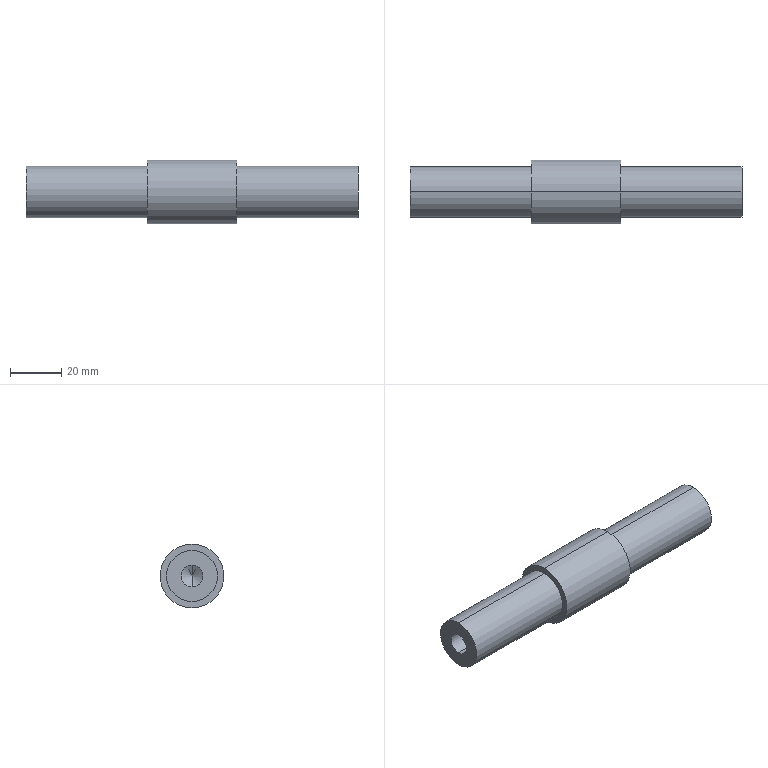Part | SolidWorks | features BaseBody 1 | 1 solid | 18 faces | box 130 x 25 x 25 mm | volume 42673 mm3 | cylinder 10 | cone 4 | plane 4 | commonest cylinder face diameters 8.5 x4 20 x4 25 x2
STEP:
#1=CARTESIAN_POINT('',(-17.5,0.,10.));
#2=VERTEX_POINT('',#1);
#3=CARTESIAN_POINT('',(-17.5,0.,-10.));
#4=VERTEX_POINT('',#3);
#5=CARTESIAN_POINT('',(-17.5,0.,0.));
#6=DIRECTION('',(-1.,0.,0.));
#7=DIRECTION('',(0.,0.,1.));
#8=AXIS2_PLACEMENT_3D('',#5,#6,#7);
#9=CIRCLE('',#8,10.);
#10=EDGE_CURVE('',#2,#4,#9,.T.);
#11=ORIENTED_EDGE('',*,*,#10,.T.);
#12=CARTESIAN_POINT('',(-65.,0.,-10.));
#13=VERTEX_POINT('',#12);
#14=CARTESIAN_POINT('',(65.,0.,-10.));
#15=DIRECTION('',(-1.,0.,0.));
#16=VECTOR('',#15,1000.);
#17=LINE('',#14,#16);
#18=EDGE_CURVE('',#4,#13,#17,.T.);
#19=ORIENTED_EDGE('',*,*,#18,.T.);
#20=CARTESIAN_POINT('',(-65.,0.,10.));
#21=VERTEX_POINT('',#20);
#22=CARTESIAN_POINT('',(-65.,0.,0.));
#23=DIRECTION('',(1.,0.,0.));
#24=DIRECTION('',(0.,0.,1.));
#25=AXIS2_PLACEMENT_3D('',#22,#23,#24);
#26=CIRCLE('',#25,10.);
#27=EDGE_CURVE('',#13,#21,#26,.T.);
#28=ORIENTED_EDGE('',*,*,#27,.T.);
#29=CARTESIAN_POINT('',(65.,0.,10.));
#30=DIRECTION('',(-1.,0.,0.));
#31=VECTOR('',#30,1000.);
#32=LINE('',#29,#31);
#33=EDGE_CURVE('',#2,#21,#32,.T.);
#34=ORIENTED_EDGE('',*,*,#33,.F.);
#35=EDGE_LOOP('',(#11,#19,#28,#34));
#36=FACE_OUTER_BOUND('',#35,.T.);
#37=CARTESIAN_POINT('',(65.,0.,0.));
#38=DIRECTION('',(-1.,0.,0.));
#39=DIRECTION('',(0.,0.,1.));
#40=AXIS2_PLACEMENT_3D('',#37,#38,#39);
#41=CYLINDRICAL_SURFACE('',#40,10.);
#42=ADVANCED_FACE('',(#36),#41,.T.);
#43=CARTESIAN_POINT('',(-27.5,0.,-4.25));
#44=VERTEX_POINT('',#43);
#45=CARTESIAN_POINT('',(-27.5,0.,4.25));
#46=VERTEX_POINT('',#45);
#47=CARTESIAN_POINT('',(-27.5,0.,0.));
#48=DIRECTION('',(-1.,0.,0.));
#49=DIRECTION('',(0.,0.,1.));
#50=AXIS2_PLACEMENT_3D('',#47,#48,#49);
#51=CIRCLE('',#50,4.25);
#52=EDGE_CURVE('',#44,#46,#51,.T.);
#53=ORIENTED_EDGE('',*,*,#52,.F.);
#54=CARTESIAN_POINT('',(-65.,0.,-4.25));
#55=VERTEX_POINT('',#54);
#56=CARTESIAN_POINT('',(-65.,0.,-4.25));
#57=DIRECTION('',(-1.,0.,0.));
#58=VECTOR('',#57,1000.);
#59=LINE('',#56,#58);
#60=EDGE_CURVE('',#44,#55,#59,.T.);
#61=ORIENTED_EDGE('',*,*,#60,.T.);
#62=CARTESIAN_POINT('',(-65.,0.,4.25));
#63=VERTEX_POINT('',#62);
#64=CARTESIAN_POINT('',(-65.,0.,0.));
#65=DIRECTION('',(-1.,0.,0.));
#66=DIRECTION('',(0.,0.,1.));
#67=AXIS2_PLACEMENT_3D('',#64,#65,#66);
#68=CIRCLE('',#67,4.25);
#69=EDGE_CURVE('',#55,#63,#68,.T.);
#70=ORIENTED_EDGE('',*,*,#69,.T.);
#71=CARTESIAN_POINT('',(-65.,0.,4.25));
#72=DIRECTION('',(-1.,0.,0.));
#73=VECTOR('',#72,1000.);
#74=LINE('',#71,#73);
#75=EDGE_CURVE('',#46,#63,#74,.T.);
#76=ORIENTED_EDGE('',*,*,#75,.F.);
#77=EDGE_LOOP('',(#53,#61,#70,#76));
#78=FACE_OUTER_BOUND('',#77,.T.);
#79=CARTESIAN_POINT('',(-65.,0.,0.));
#80=DIRECTION('',(-1.,0.,0.));
#81=DIRECTION('',(0.,0.,1.));
#82=AXIS2_PLACEMENT_3D('',#79,#80,#81);
#83=CYLINDRICAL_SURFACE('',#82,4.25);
#84=ADVANCED_FACE('',(#78),#83,.F.);
#85=CARTESIAN_POINT('',(17.5,0.,12.5));
#86=VERTEX_POINT('',#85);
#87=CARTESIAN_POINT('',(17.5,0.,-12.5));
#88=VERTEX_POINT('',#87);
#89=CARTESIAN_POINT('',(17.5,0.,0.));
#90=DIRECTION('',(-1.,0.,0.));
#91=DIRECTION('',(0.,0.,1.));
#92=AXIS2_PLACEMENT_3D('',#89,#90,#91);
#93=CIRCLE('',#92,12.5);
#94=EDGE_CURVE('',#86,#88,#93,.T.);
#95=ORIENTED_EDGE('',*,*,#94,.T.);
#96=CARTESIAN_POINT('',(-17.5,0.,-12.5));
#97=VERTEX_POINT('',#96);
#98=CARTESIAN_POINT('',(17.5,0.,-12.5));
#99=DIRECTION('',(-1.,0.,0.));
#100=VECTOR('',#99,1000.);
#101=LINE('',#98,#100);
#102=EDGE_CURVE('',#88,#97,#101,.T.);
#103=ORIENTED_EDGE('',*,*,#102,.T.);
#104=CARTESIAN_POINT('',(-17.5,0.,12.5));
#105=VERTEX_POINT('',#104);
#106=CARTESIAN_POINT('',(-17.5,0.,0.));
#107=DIRECTION('',(1.,0.,0.));
#108=DIRECTION('',(0.,0.,1.));
#109=AXIS2_PLACEMENT_3D('',#106,#107,#108);
#110=CIRCLE('',#109,12.5);
#111=EDGE_CURVE('',#97,#105,#110,.T.);
#112=ORIENTED_EDGE('',*,*,#111,.T.);
#113=CARTESIAN_POINT('',(17.5,0.,12.5));
#114=DIRECTION('',(-1.,0.,0.));
#115=VECTOR('',#114,1000.);
#116=LINE('',#113,#115);
#117=EDGE_CURVE('',#86,#105,#116,.T.);
#118=ORIENTED_EDGE('',*,*,#117,.F.);
#119=EDGE_LOOP('',(#95,#103,#112,#118));
#120=FACE_OUTER_BOUND('',#119,.T.);
#121=CARTESIAN_POINT('',(17.5,0.,0.));
#122=DIRECTION('',(-1.,0.,0.));
#123=DIRECTION('',(0.,0.,1.));
#124=AXIS2_PLACEMENT_3D('',#121,#122,#123);
#125=CYLINDRICAL_SURFACE('',#124,12.5);
#126=ADVANCED_FACE('',(#120),#125,.T.);
#127=CARTESIAN_POINT('',(-24.946,0.,0.));
#128=VERTEX_POINT('',#127);
#129=CARTESIAN_POINT('',(-27.5,0.,4.25));
#130=DIRECTION('',(-0.515,0.,0.8572));
#131=VECTOR('',#130,1000.);
#132=LINE('',#129,#131);
#133=EDGE_CURVE('',#128,#46,#132,.T.);
#134=ORIENTED_EDGE('',*,*,#133,.F.);
#135=CARTESIAN_POINT('',(-27.5,0.,-4.25));
#136=DIRECTION('',(-0.515,0.,-0.8572));
#137=VECTOR('',#136,1000.);
#138=LINE('',#135,#137);
#139=EDGE_CURVE('',#128,#44,#138,.T.);
#140=ORIENTED_EDGE('',*,*,#139,.T.);
#141=ORIENTED_EDGE('',*,*,#52,.T.);
#142=EDGE_LOOP('',(#134,#140,#141));
#143=FACE_OUTER_BOUND('',#142,.T.);
#144=CARTESIAN_POINT('',(-27.5,0.,0.));
#145=DIRECTION('',(-1.,0.,0.));
#146=DIRECTION('',(0.,0.,1.));
#147=AXIS2_PLACEMENT_3D('',#144,#145,#146);
#148=CONICAL_SURFACE('',#147,4.25,1.03);
#149=ADVANCED_FACE('',(#143),#148,.F.);
#150=CARTESIAN_POINT('',(65.,0.,10.));
#151=VERTEX_POINT('',#150);
#152=CARTESIAN_POINT('',(65.,0.,-10.));
#153=VERTEX_POINT('',#152);
#154=CARTESIAN_POINT('',(65.,0.,0.));
#155=DIRECTION('',(-1.,0.,0.));
#156=DIRECTION('',(0.,0.,1.));
#157=AXIS2_PLACEMENT_3D('',#154,#155,#156);
#158=CIRCLE('',#157,10.);
#159=EDGE_CURVE('',#151,#153,#158,.T.);
#160=ORIENTED_EDGE('',*,*,#159,.T.);
#161=CARTESIAN_POINT('',(17.5,0.,-10.));
#162=VERTEX_POINT('',#161);
#163=CARTESIAN_POINT('',(65.,0.,-10.));
#164=DIRECTION('',(-1.,0.,0.));
#165=VECTOR('',#164,1000.);
#166=LINE('',#163,#165);
#167=EDGE_CURVE('',#153,#162,#166,.T.);
#168=ORIENTED_EDGE('',*,*,#167,.T.);
#169=CARTESIAN_POINT('',(17.5,0.,10.));
#170=VERTEX_POINT('',#169);
#171=CARTESIAN_POINT('',(17.5,0.,0.));
#172=DIRECTION('',(-1.,0.,0.));
#173=DIRECTION('',(0.,0.,1.));
#174=AXIS2_PLACEMENT_3D('',#171,#172,#173);
#175=CIRCLE('',#174,10.);
#176=EDGE_CURVE('',#170,#162,#175,.T.);
#177=ORIENTED_EDGE('',*,*,#176,.F.);
#178=CARTESIAN_POINT('',(65.,0.,10.));
#179=DIRECTION('',(-1.,0.,0.));
#180=VECTOR('',#179,1000.);
#181=LINE('',#178,#180);
#182=EDGE_CURVE('',#151,#170,#181,.T.);
#183=ORIENTED_EDGE('',*,*,#182,.F.);
#184=EDGE_LOOP('',(#160,#168,#177,#183));
#185=FACE_OUTER_BOUND('',#184,.T.);
#186=CARTESIAN_POINT('',(65.,0.,0.));
#187=DIRECTION('',(-1.,0.,0.));
#188=DIRECTION('',(0.,0.,1.));
#189=AXIS2_PLACEMENT_3D('',#186,#187,#188);
#190=CYLINDRICAL_SURFACE('',#189,10.);
#191=ADVANCED_FACE('',(#185),#190,.T.);
#192=CARTESIAN_POINT('',(27.5,0.,4.25));
#193=VERTEX_POINT('',#192);
#194=CARTESIAN_POINT('',(27.5,-4.25,0.));
#195=VERTEX_POINT('',#194);
#196=CARTESIAN_POINT('',(27.5,0.,0.));
#197=DIRECTION('',(1.,0.,0.));
#198=DIRECTION('',(0.,0.,-1.));
#199=AXIS2_PLACEMENT_3D('',#196,#197,#198);
#200=CIRCLE('',#199,4.25);
#201=EDGE_CURVE('',#193,#195,#200,.T.);
#202=ORIENTED_EDGE('',*,*,#201,.F.);
#203=CARTESIAN_POINT('',(65.,0.,4.25));
#204=VERTEX_POINT('',#203);
#205=CARTESIAN_POINT('',(65.,0.,4.25));
#206=DIRECTION('',(1.,0.,0.));
#207=VECTOR('',#206,1000.);
#208=LINE('',#205,#207);
#209=EDGE_CURVE('',#193,#204,#208,.T.);
#210=ORIENTED_EDGE('',*,*,#209,.T.);
#211=CARTESIAN_POINT('',(65.,0.,-4.25));
#212=VERTEX_POINT('',#211);
#213=CARTESIAN_POINT('',(65.,0.,0.));
#214=DIRECTION('',(-1.,0.,0.));
#215=DIRECTION('',(0.,0.,-1.));
#216=AXIS2_PLACEMENT_3D('',#213,#214,#215);
#217=CIRCLE('',#216,4.25);
#218=EDGE_CURVE('',#212,#204,#217,.T.);
#219=ORIENTED_EDGE('',*,*,#218,.F.);
#220=CARTESIAN_POINT('',(27.5,0.,-4.25));
#221=VERTEX_POINT('',#220);
#222=CARTESIAN_POINT('',(65.,0.,-4.25));
#223=DIRECTION('',(1.,0.,0.));
#224=VECTOR('',#223,1000.);
#225=LINE('',#222,#224);
#226=EDGE_CURVE('',#221,#212,#225,.T.);
#227=ORIENTED_EDGE('',*,*,#226,.F.);
#228=CARTESIAN_POINT('',(27.5,0.,0.));
#229=DIRECTION('',(1.,0.,0.));
#230=DIRECTION('',(0.,0.,-1.));
#231=AXIS2_PLACEMENT_3D('',#228,#229,#230);
#232=CIRCLE('',#231,4.25);
#233=EDGE_CURVE('',#195,#221,#232,.T.);
#234=ORIENTED_EDGE('',*,*,#233,.F.);
#235=EDGE_LOOP('',(#202,#210,#219,#227,#234));
#236=FACE_OUTER_BOUND('',#235,.T.);
#237=CARTESIAN_POINT('',(65.,0.,0.));
#238=DIRECTION('',(1.,0.,0.));
#239=DIRECTION('',(0.,0.,-1.));
#240=AXIS2_PLACEMENT_3D('',#237,#238,#239);
#241=CYLINDRICAL_SURFACE('',#240,4.25);
#242=ADVANCED_FACE('',(#236),#241,.F.);
#243=CARTESIAN_POINT('',(24.946,0.,0.));
#244=VERTEX_POINT('',#243);
#245=CARTESIAN_POINT('',(27.5,4.25,0.));
#246=VERTEX_POINT('',#245);
#247=CARTESIAN_POINT('',(27.5,4.25,0.));
#248=DIRECTION('',(0.515,0.8572,0.));
#249=VECTOR('',#248,1000.);
#250=LINE('',#247,#249);
#251=EDGE_CURVE('',#244,#246,#250,.T.);
#252=ORIENTED_EDGE('',*,*,#251,.F.);
#253=CARTESIAN_POINT('',(27.5,-4.25,0.));
#254=DIRECTION('',(0.515,-0.8572,0.));
#255=VECTOR('',#254,1000.);
#256=LINE('',#253,#255);
#257=EDGE_CURVE('',#244,#195,#256,.T.);
#258=ORIENTED_EDGE('',*,*,#257,.T.);
#259=ORIENTED_EDGE('',*,*,#233,.T.);
#260=CARTESIAN_POINT('',(27.5,0.,0.));
#261=DIRECTION('',(1.,0.,0.));
#262=DIRECTION('',(0.,0.,-1.));
#263=AXIS2_PLACEMENT_3D('',#260,#261,#262);
#264=CIRCLE('',#263,4.25);
#265=EDGE_CURVE('',#221,#246,#264,.T.);
#266=ORIENTED_EDGE('',*,*,#265,.T.);
#267=EDGE_LOOP('',(#252,#258,#259,#266));
#268=FACE_OUTER_BOUND('',#267,.T.);
#269=CARTESIAN_POINT('',(27.5,0.,0.));
#270=DIRECTION('',(1.,0.,0.));
#271=DIRECTION('',(0.,1.,0.));
#272=AXIS2_PLACEMENT_3D('',#269,#270,#271);
#273=CONICAL_SURFACE('',#272,4.25,1.03);
#274=ADVANCED_FACE('',(#268),#273,.F.);
#275=ORIENTED_EDGE('',*,*,#18,.F.);
#276=CARTESIAN_POINT('',(-17.5,0.,0.));
#277=DIRECTION('',(-1.,0.,0.));
#278=DIRECTION('',(0.,0.,1.));
#279=AXIS2_PLACEMENT_3D('',#276,#277,#278);
#280=CIRCLE('',#279,10.);
#281=EDGE_CURVE('',#4,#2,#280,.T.);
#282=ORIENTED_EDGE('',*,*,#281,.T.);
#283=ORIENTED_EDGE('',*,*,#33,.T.);
#284=CARTESIAN_POINT('',(-65.,0.,0.));
#285=DIRECTION('',(1.,0.,0.));
#286=DIRECTION('',(0.,0.,1.));
#287=AXIS2_PLACEMENT_3D('',#284,#285,#286);
#288=CIRCLE('',#287,10.);
#289=EDGE_CURVE('',#21,#13,#288,.T.);
#290=ORIENTED_EDGE('',*,*,#289,.T.);
#291=EDGE_LOOP('',(#275,#282,#283,#290));
#292=FACE_OUTER_BOUND('',#291,.T.);
#293=CARTESIAN_POINT('',(65.,0.,0.));
#294=DIRECTION('',(-1.,0.,0.));
#295=DIRECTION('',(0.,0.,1.));
#296=AXIS2_PLACEMENT_3D('',#293,#294,#295);
#297=CYLINDRICAL_SURFACE('',#296,10.);
#298=ADVANCED_FACE('',(#292),#297,.T.);
#299=ORIENTED_EDGE('',*,*,#289,.F.);
#300=ORIENTED_EDGE('',*,*,#27,.F.);
#301=EDGE_LOOP('',(#299,#300));
#302=FACE_OUTER_BOUND('',#301,.T.);
#303=CARTESIAN_POINT('',(-65.,0.,0.));
#304=DIRECTION('',(-1.,0.,0.));
#305=DIRECTION('',(0.,0.,1.));
#306=AXIS2_PLACEMENT_3D('',#303,#304,#305);
#307=CIRCLE('',#306,4.25);
#308=EDGE_CURVE('',#63,#55,#307,.T.);
#309=ORIENTED_EDGE('',*,*,#308,.F.);
#310=ORIENTED_EDGE('',*,*,#69,.F.);
#311=EDGE_LOOP('',(#309,#310));
#312=FACE_BOUND('',#311,.T.);
#313=CARTESIAN_POINT('',(-65.,0.,0.));
#314=DIRECTION('',(1.,0.,0.));
#315=DIRECTION('',(0.,0.,-1.));
#316=AXIS2_PLACEMENT_3D('',#313,#314,#315);
#317=PLANE('',#316);
#318=ADVANCED_FACE('',(#302,#312),#317,.F.);
#319=CARTESIAN_POINT('',(-17.5,0.,0.));
#320=DIRECTION('',(1.,0.,0.));
#321=DIRECTION('',(0.,0.,1.));
#322=AXIS2_PLACEMENT_3D('',#319,#320,#321);
#323=CIRCLE('',#322,12.5);
#324=EDGE_CURVE('',#105,#97,#323,.T.);
#325=ORIENTED_EDGE('',*,*,#324,.F.);
#326=ORIENTED_EDGE('',*,*,#111,.F.);
#327=EDGE_LOOP('',(#325,#326));
#328=FACE_OUTER_BOUND('',#327,.T.);
#329=ORIENTED_EDGE('',*,*,#10,.F.);
#330=ORIENTED_EDGE('',*,*,#281,.F.);
#331=EDGE_LOOP('',(#329,#330));
#332=FACE_BOUND('',#331,.T.);
#333=CARTESIAN_POINT('',(-17.5,0.,0.));
#334=DIRECTION('',(1.,0.,0.));
#335=DIRECTION('',(0.,0.,-1.));
#336=AXIS2_PLACEMENT_3D('',#333,#334,#335);
#337=PLANE('',#336);
#338=ADVANCED_FACE('',(#328,#332),#337,.F.);
#339=ORIENTED_EDGE('',*,*,#60,.F.);
#340=CARTESIAN_POINT('',(-27.5,0.,0.));
#341=DIRECTION('',(-1.,0.,0.));
#342=DIRECTION('',(0.,0.,1.));
#343=AXIS2_PLACEMENT_3D('',#340,#341,#342);
#344=CIRCLE('',#343,4.25);
#345=EDGE_CURVE('',#46,#44,#344,.T.);
#346=ORIENTED_EDGE('',*,*,#345,.F.);
#347=ORIENTED_EDGE('',*,*,#75,.T.);
#348=ORIENTED_EDGE('',*,*,#308,.T.);
#349=EDGE_LOOP('',(#339,#346,#347,#348));
#350=FACE_OUTER_BOUND('',#349,.T.);
#351=CARTESIAN_POINT('',(-65.,0.,0.));
#352=DIRECTION('',(-1.,0.,0.));
#353=DIRECTION('',(0.,0.,1.));
#354=AXIS2_PLACEMENT_3D('',#351,#352,#353);
#355=CYLINDRICAL_SURFACE('',#354,4.25);
#356=ADVANCED_FACE('',(#350),#355,.F.);
#357=ORIENTED_EDGE('',*,*,#102,.F.);
#358=CARTESIAN_POINT('',(17.5,0.,0.));
#359=DIRECTION('',(-1.,0.,0.));
#360=DIRECTION('',(0.,0.,1.));
#361=AXIS2_PLACEMENT_3D('',#358,#359,#360);
#362=CIRCLE('',#361,12.5);
#363=EDGE_CURVE('',#88,#86,#362,.T.);
#364=ORIENTED_EDGE('',*,*,#363,.T.);
#365=ORIENTED_EDGE('',*,*,#117,.T.);
#366=ORIENTED_EDGE('',*,*,#324,.T.);
#367=EDGE_LOOP('',(#357,#364,#365,#366));
#368=FACE_OUTER_BOUND('',#367,.T.);
#369=CARTESIAN_POINT('',(17.5,0.,0.));
#370=DIRECTION('',(-1.,0.,0.));
#371=DIRECTION('',(0.,0.,1.));
#372=AXIS2_PLACEMENT_3D('',#369,#370,#371);
#373=CYLINDRICAL_SURFACE('',#372,12.5);
#374=ADVANCED_FACE('',(#368),#373,.T.);
#375=ORIENTED_EDGE('',*,*,#139,.F.);
#376=ORIENTED_EDGE('',*,*,#133,.T.);
#377=ORIENTED_EDGE('',*,*,#345,.T.);
#378=EDGE_LOOP('',(#375,#376,#377));
#379=FACE_OUTER_BOUND('',#378,.T.);
#380=CARTESIAN_POINT('',(-27.5,0.,0.));
#381=DIRECTION('',(-1.,0.,0.));
#382=DIRECTION('',(0.,0.,1.));
#383=AXIS2_PLACEMENT_3D('',#380,#381,#382);
#384=CONICAL_SURFACE('',#383,4.25,1.03);
#385=ADVANCED_FACE('',(#379),#384,.F.);
#386=ORIENTED_EDGE('',*,*,#94,.F.);
#387=ORIENTED_EDGE('',*,*,#363,.F.);
#388=EDGE_LOOP('',(#386,#387));
#389=FACE_OUTER_BOUND('',#388,.T.);
#390=ORIENTED_EDGE('',*,*,#176,.T.);
#391=CARTESIAN_POINT('',(17.5,0.,0.));
#392=DIRECTION('',(-1.,0.,0.));
#393=DIRECTION('',(0.,0.,1.));
#394=AXIS2_PLACEMENT_3D('',#391,#392,#393);
#395=CIRCLE('',#394,10.);
#396=EDGE_CURVE('',#162,#170,#395,.T.);
#397=ORIENTED_EDGE('',*,*,#396,.T.);
#398=EDGE_LOOP('',(#390,#397));
#399=FACE_BOUND('',#398,.T.);
#400=CARTESIAN_POINT('',(17.5,0.,0.));
#401=DIRECTION('',(1.,0.,0.));
#402=DIRECTION('',(0.,0.,-1.));
#403=AXIS2_PLACEMENT_3D('',#400,#401,#402);
#404=PLANE('',#403);
#405=ADVANCED_FACE('',(#389,#399),#404,.T.);
#406=ORIENTED_EDGE('',*,*,#167,.F.);
#407=CARTESIAN_POINT('',(65.,0.,0.));
#408=DIRECTION('',(-1.,0.,0.));
#409=DIRECTION('',(0.,0.,1.));
#410=AXIS2_PLACEMENT_3D('',#407,#408,#409);
#411=CIRCLE('',#410,10.);
#412=EDGE_CURVE('',#153,#151,#411,.T.);
#413=ORIENTED_EDGE('',*,*,#412,.T.);
#414=ORIENTED_EDGE('',*,*,#182,.T.);
#415=ORIENTED_EDGE('',*,*,#396,.F.);
#416=EDGE_LOOP('',(#406,#413,#414,#415));
#417=FACE_OUTER_BOUND('',#416,.T.);
#418=CARTESIAN_POINT('',(65.,0.,0.));
#419=DIRECTION('',(-1.,0.,0.));
#420=DIRECTION('',(0.,0.,1.));
#421=AXIS2_PLACEMENT_3D('',#418,#419,#420);
#422=CYLINDRICAL_SURFACE('',#421,10.);
#423=ADVANCED_FACE('',(#417),#422,.T.);
#424=ORIENTED_EDGE('',*,*,#159,.F.);
#425=ORIENTED_EDGE('',*,*,#412,.F.);
#426=EDGE_LOOP('',(#424,#425));
#427=FACE_OUTER_BOUND('',#426,.T.);
#428=ORIENTED_EDGE('',*,*,#218,.T.);
#429=CARTESIAN_POINT('',(65.,0.,0.));
#430=DIRECTION('',(-1.,0.,0.));
#431=DIRECTION('',(0.,0.,-1.));
#432=AXIS2_PLACEMENT_3D('',#429,#430,#431);
#433=CIRCLE('',#432,4.25);
#434=EDGE_CURVE('',#204,#212,#433,.T.);
#435=ORIENTED_EDGE('',*,*,#434,.T.);
#436=EDGE_LOOP('',(#428,#435));
#437=FACE_BOUND('',#436,.T.);
#438=CARTESIAN_POINT('',(65.,0.,0.));
#439=DIRECTION('',(1.,0.,0.));
#440=DIRECTION('',(0.,0.,-1.));
#441=AXIS2_PLACEMENT_3D('',#438,#439,#440);
#442=PLANE('',#441);
#443=ADVANCED_FACE('',(#427,#437),#442,.T.);
#444=ORIENTED_EDGE('',*,*,#209,.F.);
#445=CARTESIAN_POINT('',(27.5,0.,0.));
#446=DIRECTION('',(1.,0.,0.));
#447=DIRECTION('',(0.,0.,-1.));
#448=AXIS2_PLACEMENT_3D('',#445,#446,#447);
#449=CIRCLE('',#448,4.25);
#450=EDGE_CURVE('',#246,#193,#449,.T.);
#451=ORIENTED_EDGE('',*,*,#450,.F.);
#452=ORIENTED_EDGE('',*,*,#265,.F.);
#453=ORIENTED_EDGE('',*,*,#226,.T.);
#454=ORIENTED_EDGE('',*,*,#434,.F.);
#455=EDGE_LOOP('',(#444,#451,#452,#453,#454));
#456=FACE_OUTER_BOUND('',#455,.T.);
#457=CARTESIAN_POINT('',(65.,0.,0.));
#458=DIRECTION('',(1.,0.,0.));
#459=DIRECTION('',(0.,0.,-1.));
#460=AXIS2_PLACEMENT_3D('',#457,#458,#459);
#461=CYLINDRICAL_SURFACE('',#460,4.25);
#462=ADVANCED_FACE('',(#456),#461,.F.);
#463=ORIENTED_EDGE('',*,*,#257,.F.);
#464=ORIENTED_EDGE('',*,*,#251,.T.);
#465=ORIENTED_EDGE('',*,*,#450,.T.);
#466=ORIENTED_EDGE('',*,*,#201,.T.);
#467=EDGE_LOOP('',(#463,#464,#465,#466));
#468=FACE_OUTER_BOUND('',#467,.T.);
#469=CARTESIAN_POINT('',(27.5,0.,0.));
#470=DIRECTION('',(1.,0.,0.));
#471=DIRECTION('',(0.,1.,0.));
#472=AXIS2_PLACEMENT_3D('',#469,#470,#471);
#473=CONICAL_SURFACE('',#472,4.25,1.03);
#474=ADVANCED_FACE('',(#468),#473,.F.);
#475=CLOSED_SHELL('',(#42,#84,#126,#149,#191,#242,#274,#298,#318,#338,#356,#374,#385,#405,#423,#443,#462,#474));
#476=MANIFOLD_SOLID_BREP('',#475);
#477=CARTESIAN_POINT('',(0.,0.,0.));
#478=DIRECTION('',(0.,0.,1.));
#479=DIRECTION('',(1.,0.,0.));
#480=AXIS2_PLACEMENT_3D('',#477,#478,#479);
#481=(LENGTH_UNIT()NAMED_UNIT(*)SI_UNIT(.MILLI.,.METRE.));
#482=UNCERTAINTY_MEASURE_WITH_UNIT(LENGTH_MEASURE(0.00001),#481,'','');
#483=(NAMED_UNIT(*)PLANE_ANGLE_UNIT()SI_UNIT($,.RADIAN.));
#484=(NAMED_UNIT(*)SI_UNIT($,.STERADIAN.)SOLID_ANGLE_UNIT());
#485=(GEOMETRIC_REPRESENTATION_CONTEXT(3)GLOBAL_UNCERTAINTY_ASSIGNED_CONTEXT((#482))GLOBAL_UNIT_ASSIGNED_CONTEXT((#481,#483,#484))REPRESENTATION_CONTEXT('',''));
#486=ADVANCED_BREP_SHAPE_REPRESENTATION('',(#476,#480),#485);